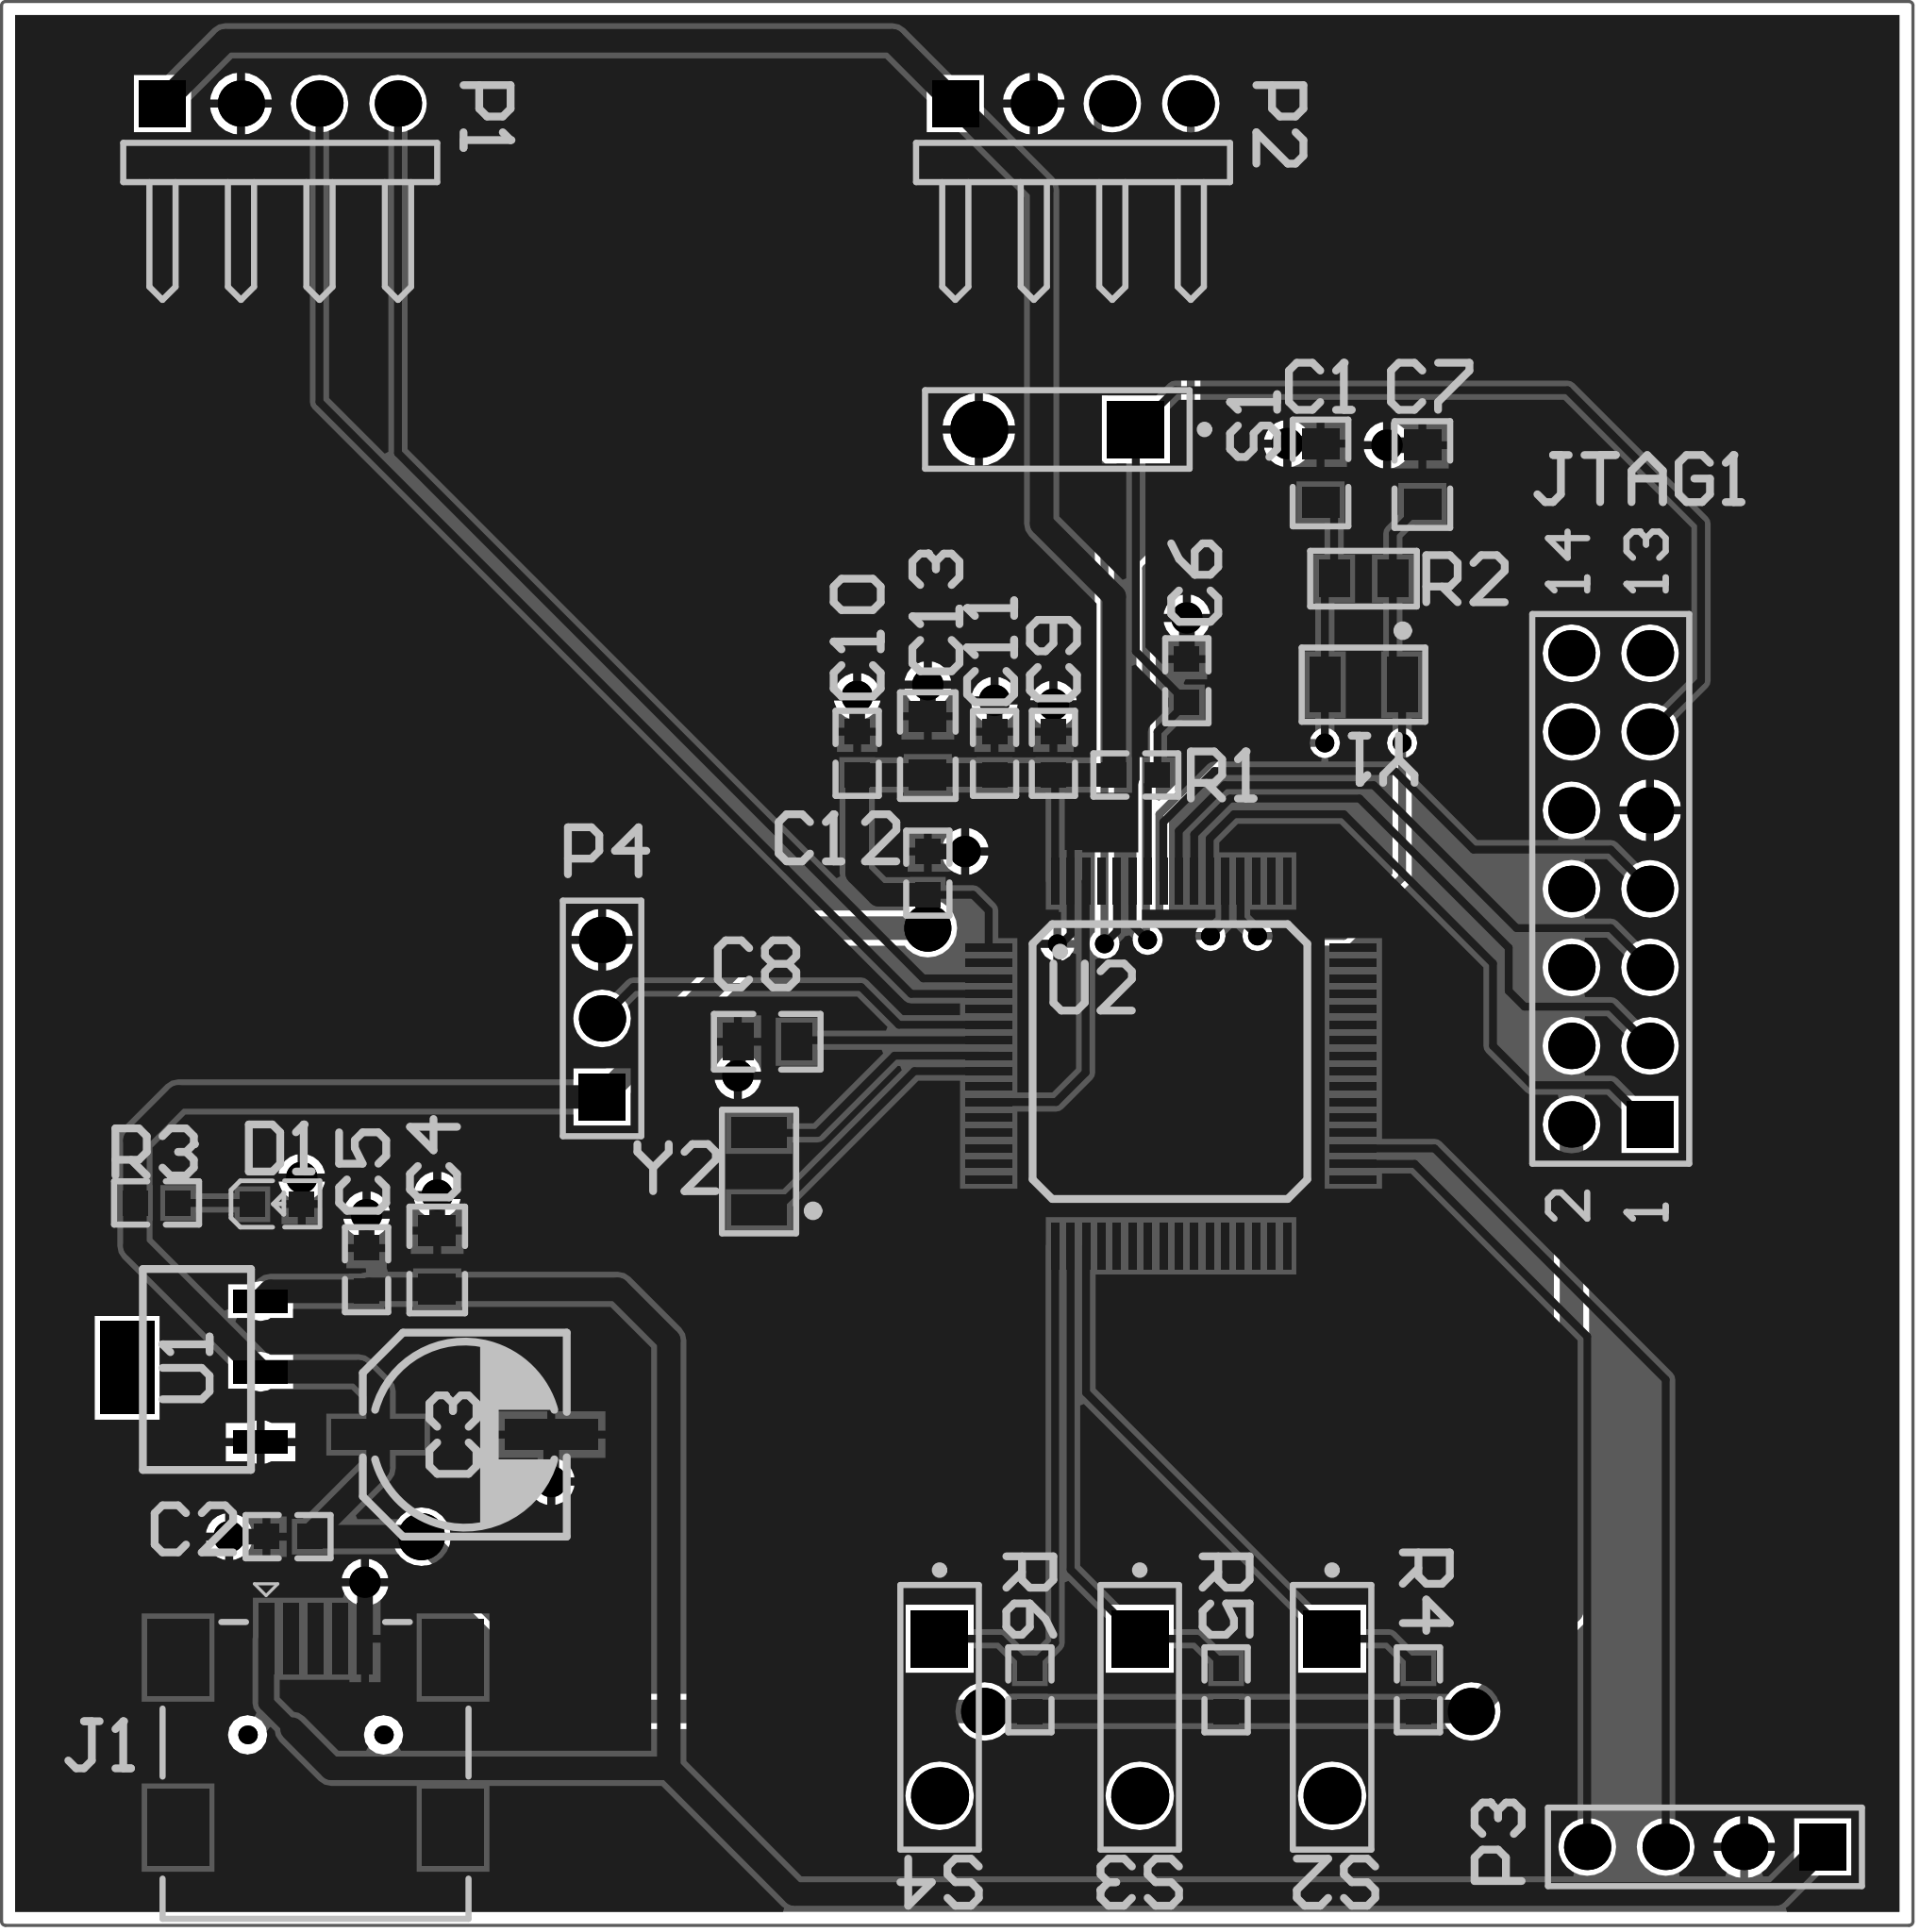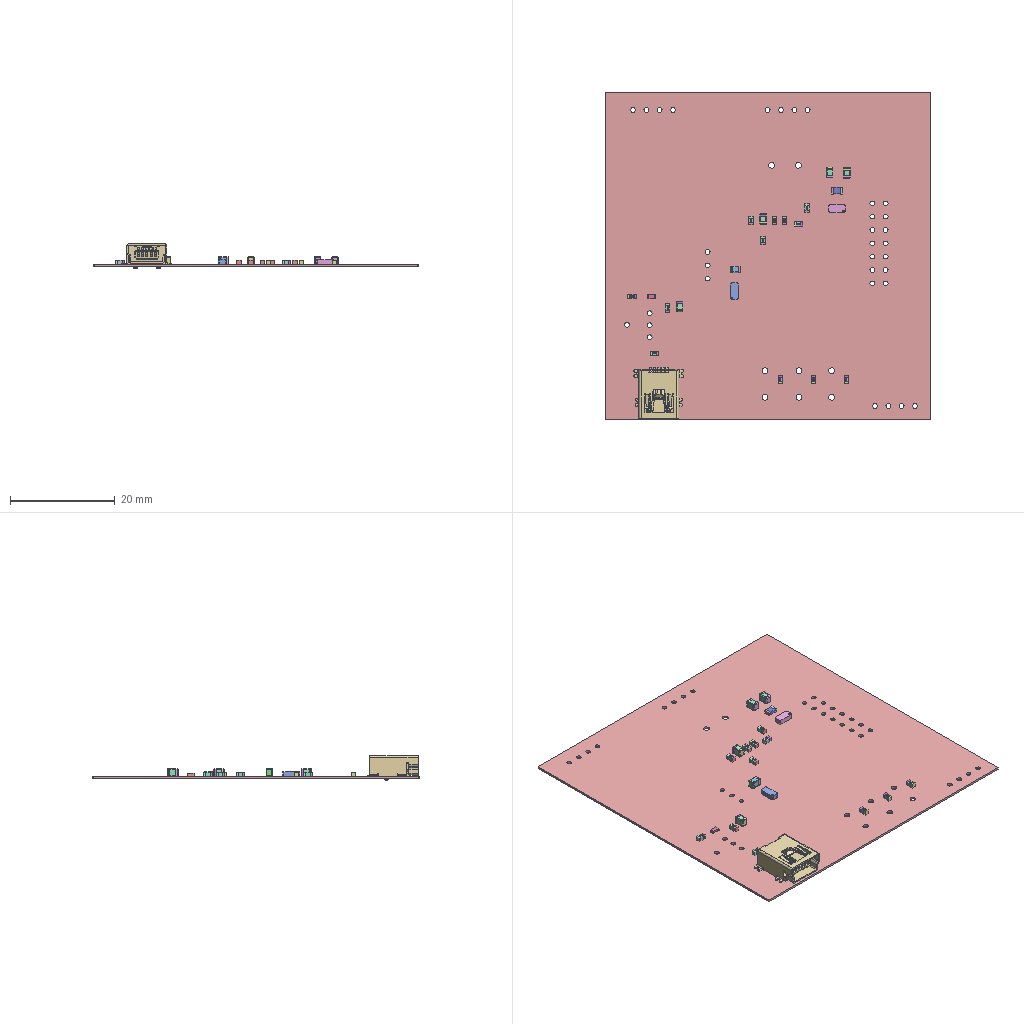Circuit board layout | Altium Designer | box 61.8 x 62.2 x 4.6 mm
Layer stack:
# Altium Designer layer stack of  (unit mm; dielectric type: 0 none, 1 core, 2 prepreg, 3 surface material)
index,name,kind,layer,copper_thickness_mm,dielectric_type,dielectric_thickness_mm,dielectric_material,dielectric_constant
0,Top Paste,other,,,,,,
1,Top Overlay,other,,,,,,
2,Top Solder,dielectric,,,3,0.0102,Solder Resist,3.5
3,Top Layer,copper,Top Layer,0.0356,,,,
4,Dielectric 1,dielectric,,,0,0.32,FR-4,4.8
5,Bottom Layer,copper,Bottom Layer,0.0356,,,,
6,Bottom Solder,dielectric,,,3,0.0102,Solder Resist,3.5
7,Bottom Overlay,other,,,,,,
8,Bottom Paste,other,,,,,,
# drill layer pairs: low layer,high layer
drill_pair,Top Layer,Bottom Layer
Part placement:
Designator,Comment,Layer,Footprint,Center-X(mm),Center-Y(mm),Rotation
Y2,32768,TopLayer,XTAL-SMD-NX3215SA-32.768K-STD-MUS-2,102.489,61.341,90
Y1,8M,TopLayer,XTAL-SMD-NX3215SA-32.768K-STD-MUS-2,122.047,77.089,180
U2,MSP430F149,TopLayer,MSP430F149,115.82,64.839,360
U1,AMS1117-3.3,TopLayer,AMS1117-3.3,84.201,54.87,90
S4,SW-PB,TopLayer,SPST-2,108.331,43.688,270
S3,SW-PB,TopLayer,SPST-2,114.808,43.688,270
S2,SW-PB,TopLayer,SPST-2,121.031,43.688,270
S1,SW-SPST,TopLayer,SPST-2,112.141,85.344,180
R6,10K,TopLayer,0603R,111.252,44.577,270
R5,10K,TopLayer,0603R,117.602,44.577,270
R4,10K,TopLayer,0603R,123.825,44.577,270
R3,510R,TopLayer,0603R,82.993,60.325,180
R2,RC-1M,TopLayer,0805R,122.047,80.518,180
R1,10K,TopLayer,0603R,114.681,74.168,180
P4,Buzzer,TopLayer,HDR1X3,97.409,66.294,90
P3,Bluetooth module,TopLayer,HDR1X4,133.096,39.497,180
P2,BMP108,TopLayer,HDR1X4H,112.649,95.885,360
P1,OLED,TopLayer,HDR1X4H,86.995,95.885,360
JTAG1,DIP14,TopLayer,HDR2X7,130.048,70.485,90
J1,Mini-USB,TopLayer,USB-MINI-A,88.138,43.174,360
D1,LED0,TopLayer,LED0603-RD,86.891,60.287,360
C13,106,TopLayer,0805C,107.95,75.118,90
C12,104,TopLayer,0603C,107.95,70.993,90
C11,104,TopLayer,0603C,110.109,74.868,90
C10,104,TopLayer,0603C,105.664,74.868,90
C9,104,TopLayer,0603C,112.014,74.868,90
C8,S0805-20P,TopLayer,0805C,102.753,65.539,0
C7,S0805-20P,TopLayer,0805C,123.952,83.886,270
C6,104,TopLayer,0603C,116.332,77.216,90
C5,104,TopLayer,0603C,89.789,58.166,90
C4,10uF,TopLayer,0805C,92.075,58.481,90
C3,10uF,TopLayer,贴片电容,92.964,52.832,270
C2,104,TopLayer,0603C,87.249,49.53,180
C1,S0805-20P,TopLayer,0805C,120.657,83.937,270
Pad and via stacks:
# Altium Designer via and pad stacks of  (unit mm). Each distinct definition once, with the count of objects using it.
# via: kind,start_layer,end_layer,hole_mm,diameter_mm,mode(0 simple;1 top-mid-bottom;2 full stack),diameter_per_layer,count,example_net
# pad: kind,layer,hole_mm,hole_type(0 round;1 square;2 slot),plating,top_size,top_shape(1 round;2 rect;3 octagon;9 rounded rect),mid_size,bottom_size,mode,footprint,size_per_layer,count,example
pad,Top Layer,0,0,plated,2x2.5,2,2x2.5,2x2.5,0,USB-MINI-A,,4,J1.0
pad,Top Layer,0,0,plated,0.5x2.3,2,0.5x2.3,0.5x2.3,0,USB-MINI-A,,5,J1.1
pad,Top Layer,0,0,plated,0.8x0.8,2,0.8x0.8,0.8x0.8,0,0603R,,10,R1.1
pad,Top Layer,0,0,plated,1x1.2,2,1x1.2,1x1.2,0,0805C,,10,C1.2
pad,Top Layer,0,0,plated,0.8x0.8,2,0.8x0.8,0.8x0.8,0,0603C,,14,C2.2
pad,Top Layer,0,0,plated,3x1,2,3x1,3x1,0,\u00CC\u00F9\u00C6\u00AC\u00B5\u00E7\u00C8\u00DD,,2,C3.2
pad,Top Layer,0,0,plated,1x1.2,2,1x1.2,1x1.2,0,0805R,,2,R2.1
pad,Top Layer,0,0,unplated,1x1.8,2,1x1.8,1x1.8,0,XTAL-SMD-NX3215SA-32.768K-STD-MUS-2,,4,Y1.1
pad,Top Layer,0,0,plated,0.8x0.8,2,0.8x0.8,0.8x0.8,0,LED0603-RD,,2,D1.2
pad,Top Layer,0,0,plated,1.5x0.25,2,1.5x0.25,1.5x0.25,0,MSP430F149,,64,U2.2
pad,Multi-Layer,0.9144,0,plated,3x1.75,2,3x1.75,3x1.75,0,AMS1117-3.3,,1,U1.4
pad,Multi-Layer,0.9144,0,plated,0.74x1.75,2,0.74x1.75,0.74x1.75,0,AMS1117-3.3,,3,U1.3
pad,Multi-Layer,0.9,0,unplated,0.6x0.6,1,0.6x0.6,0.6x0.6,0,USB-MINI-A,,2,J1.MH1
pad,Multi-Layer,0.9,0,plated,1.5x1.5,2,1.5x1.5,1.5x1.5,0,HDR2X7,,1,JTAG1.1
pad,Multi-Layer,0.9,0,plated,1.5x1.5,1,1.5x1.5,1.5x1.5,0,HDR2X7,,13,JTAG1.2
pad,Multi-Layer,1.1,0,plated,1.85x1.85,2,1.85x1.85,1.85x1.85,0,SPST-2,,4,S1.1
pad,Multi-Layer,1.1,0,plated,1.85x1.85,1,1.85x1.85,1.85x1.85,0,SPST-2,,4,S1.2
pad,Multi-Layer,0.9,0,plated,1.5x1.5,1,1.5x1.5,1.5x1.5,0,HDR1X4H,,6,P1.4
pad,Multi-Layer,0.9,0,plated,1.5x1.5,2,1.5x1.5,1.5x1.5,0,HDR1X4H,,2,P1.1
pad,Multi-Layer,0.9,0,plated,1.5x1.5,1,1.5x1.5,1.5x1.5,0,HDR1X4,,3,P3.4
pad,Multi-Layer,0.9,0,plated,1.5x1.5,2,1.5x1.5,1.5x1.5,0,HDR1X4,,1,P3.1
pad,Multi-Layer,0.9,0,plated,1.5x1.5,2,1.5x1.5,1.5x1.5,0,HDR1X3,,1,P4.1
pad,Multi-Layer,0.9,0,plated,1.5x1.5,1,1.5x1.5,1.5x1.5,0,HDR1X3,,2,P4.2
via,Top Layer,Bottom Layer,0.3048,0.6096,0,,7,GND
via,Top Layer,Bottom Layer,0.508,1.016,0,,15,GND
via,Top Layer,Bottom Layer,0.762,1.524,0,,4,3V3
Copper pours:
name,layer,net,type(0 solid;1 hatched;2 none)
G,Top Layer,GND,0
G,Bottom Layer,GND,0
Design rules, without the lines most boards share:
# Altium Designer design rules of  (exported by Altium Designer, unit mm)
# columns: name | kind | enabled | priority | scope1 | scope2 | descriptor | typed fields (field=value)
SilkToSilkClearance | 55 | enabled | 1 | All | All | Silk to Silk (Clearance=0mil) (All),(All) |
SilkToSolderMaskClearance | 54 | enabled | 1 | IsPad | All | Silk To Solder Mask (Clearance=0mil) (IsPad),(All) |
MinimumSolderMaskSliver | 53 | enabled | 1 | All | All | Minimum Solder Mask Sliver (Gap=0mil) (All),(All) |
HoleToHoleClearance | 52 | enabled | 1 | All | All | Hole To Hole Clearance (Gap=10mil) (All),(All) | gap=0.254
DiffPairsRouting | 51 | enabled | 1 | All | All | Differential Pairs Uncoupled Length using the Gap Constraints (Min=10mil) (Max=10mil) (Prefered=10mil)  and Width Constraints (Min=15mil) (Max=15mil) (Prefered=15mil) (All) |
SolderMaskExpansion | 13 | enabled | 1 | All | All | Solder Mask Expansion (Expansion =4mil) (All) | expansion=0.1016
PasteMaskExpansion | 14 | enabled | 1 | All | All | Paste Mask Expansion (Expansion =0mil) (All) | expansion=0
RoutingVias | 11 | enabled | 1 | All | All | Routing Via (MinHoleWidth=28mil) (MaxHoleWidth=28mil) (PreferredHoleWidth=28mil) (MinWidth=50mil) (MaxWidth=50mil) (PreferedWidth=50mil) (All) | via_min_hole=0.7112 via_max_hole=0.7112 via_preferred_diameter=1.27 via_preferred_hole=0.7112
Width | 2 | enabled | 1 | All | All | Width Constraint (Min=10mil) (Max=30mil) (Preferred=10mil) (All) |
PolygonConnect | 20 | enabled | 1 | All | All | Polygon Connect Rule(Relief Connect )(Conductor Width=10mil) (Relief Angle=90 Angle) (Entries=4) (Air Gap Width=10mil) (All),(All) | connect_style(0=relief,1=direct,2=none)=0 relief_conductor_width=0.254 relief_entries=4
PlaneConnect | 6 | enabled | 1 | All | All | Power Plane Connect Rule(Relief Connect )(Expansion=20mil) (Conductor Width=10mil) (Air Gap=10mil) (Entries=4) (All) | relief_conductor_width=0.254 relief_entries=4 relief_expansion=0.508
Clearance | 0 | enabled | 1 | All | All | Clearance Constraint (Gap=7mil) (All),(All) | gap=0.1778
Classes set for this board:
# Altium Designer classes of  (member kind: 0 net, 1 component, 2 from-to, 3 pad, 4 layer, 5 differential pair, 6 design channel, 7 polygon, 8 structure, 9 xSignal)
# columns: class name | member kind | superclass | members
msp430 | 1 | no | C1; C2; C3; C4; C5; C6; C7; C8; C9; C10; C11; C12; C13; D1; J1; JTAG1; P1; P2; P3; P4; R1; R2; R3; R4; R5; R6; S1; S2; S3; S4; U1; U2; Y1; Y2;